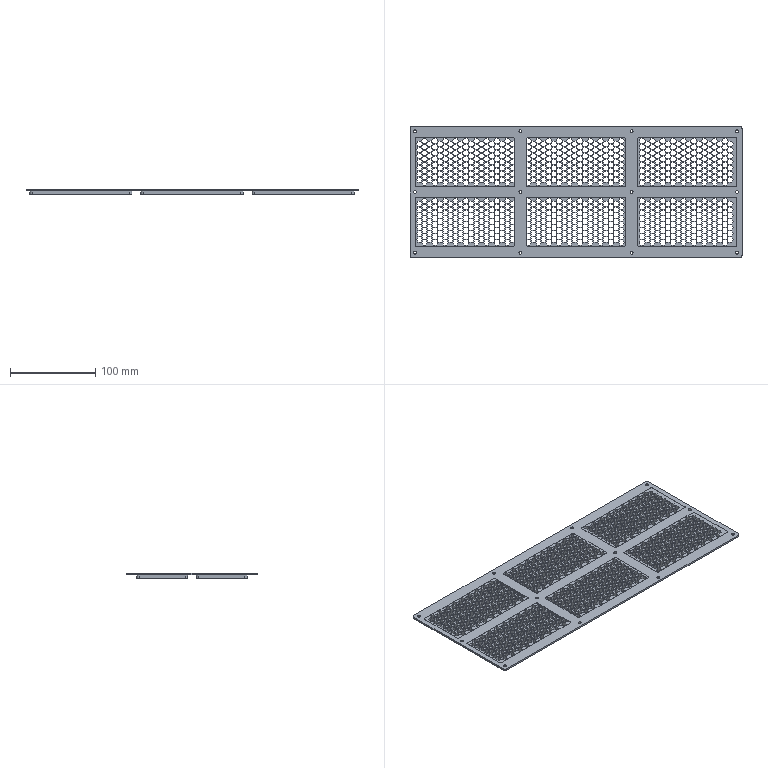NC program | NX | posted with a generic post
Whole program:
N10 G17 G21 G94 G90
(DRILLING_5 , TOOL : D4_CHAMFER)
N12 T04 M6
N14 G54
N16 G17 G0 G90 X188.5 Y-71. S0 M3
N18 G43 Z20. H4
N20 G94 G81 G98 Z-8.1 F250. R-3.5
N22 Y0.
N24 Y71.
N26 X65.
N28 Y0.
N30 Y-71.
N32 X-65.
N34 Y0.
N36 Y71.
N38 X-188.5
N40 Y0.
N42 Y-71.
N44 G80
N46 G0 X-188.5 Y-71. Z20.
N48 M5
(DRILLING_5_COPY , TOOL : Z2.5)
N50 T09 M6
N52 G54
N54 G17 G0 G90 X188.5 Y-71. S3000 M3
N56 G43 Z20. H9
N58 G94 G83 G98 Z-18.5 F150. Q2. R-3.5
N60 Y0.
N62 Y71.
N64 X65.
N66 Y0.
N68 Y-71.
N70 X-65.
N72 Y0.
N74 Y71.
N76 X-188.5
N78 Y0.
N80 Y-71.
N82 G80
N84 G0 X-188.5 Y-71. Z20.
N86 M5
(DRILLING_5_COPY_COPY , TOOL : M3X0.5)
N88 T10 M6
N90 G54
N92 G17 G0 G90 X188.5 Y-71. S300 M3
N94 G43 Z20. H10
N96 G84 G94 G98 Z-13.5 F150. R-3.5
N98 Y0.
N100 Y71.
N102 X65.
N104 Y0.
N106 Y-71.
N108 X-65.
N110 Y0.
N112 Y71.
N114 X-188.5
N116 Y0.
N118 Y-71.
N120 G80
N122 G0 X-188.5 Y-71. Z20.
N124 M5
N126 M2